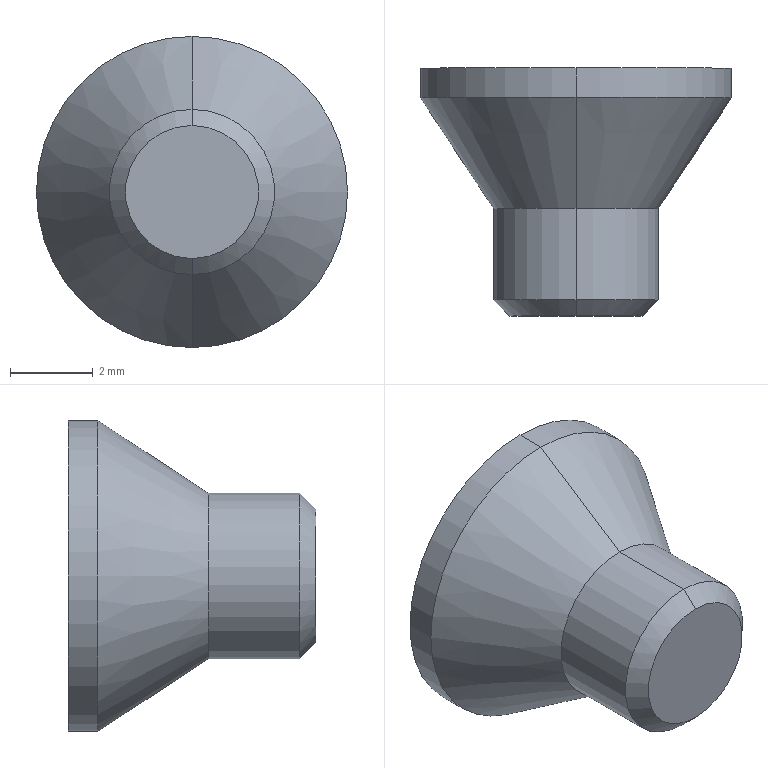Part | SolidWorks | features BaseBody 1 | 1 solid | 17 faces | box 7.53 x 6 x 7.53 mm | volume 127.383 mm3 | plane 9 | cone 4 | cylinder 4 | commonest cylinder face diameters 4 x2 7.53 x2
STEP:
#1=CARTESIAN_POINT('',(0.,-2.6,-1.61));
#2=VERTEX_POINT('',#1);
#3=CARTESIAN_POINT('',(0.,-2.6,1.61));
#4=VERTEX_POINT('',#3);
#5=CARTESIAN_POINT('',(0.,-2.6,0.));
#6=DIRECTION('',(0.,-1.,0.));
#7=DIRECTION('',(0.,0.,-1.));
#8=AXIS2_PLACEMENT_3D('',#5,#6,#7);
#9=CIRCLE('',#8,1.61);
#10=EDGE_CURVE('',#2,#4,#9,.T.);
#11=ORIENTED_EDGE('',*,*,#10,.F.);
#12=CARTESIAN_POINT('',(0.,-2.21,-2.));
#13=VERTEX_POINT('',#12);
#14=CARTESIAN_POINT('',(0.,-2.6,-1.61));
#15=DIRECTION('',(0.,0.7071,-0.7071));
#16=VECTOR('',#15,1000.);
#17=LINE('',#14,#16);
#18=EDGE_CURVE('',#2,#13,#17,.T.);
#19=ORIENTED_EDGE('',*,*,#18,.T.);
#20=CARTESIAN_POINT('',(0.,-2.21,2.));
#21=VERTEX_POINT('',#20);
#22=CARTESIAN_POINT('',(0.,-2.21,0.));
#23=DIRECTION('',(0.,1.,0.));
#24=DIRECTION('',(0.,0.,-1.));
#25=AXIS2_PLACEMENT_3D('',#22,#23,#24);
#26=CIRCLE('',#25,2.);
#27=EDGE_CURVE('',#21,#13,#26,.T.);
#28=ORIENTED_EDGE('',*,*,#27,.F.);
#29=CARTESIAN_POINT('',(0.,-2.6,1.61));
#30=DIRECTION('',(0.,0.7071,0.7071));
#31=VECTOR('',#30,1000.);
#32=LINE('',#29,#31);
#33=EDGE_CURVE('',#4,#21,#32,.T.);
#34=ORIENTED_EDGE('',*,*,#33,.F.);
#35=EDGE_LOOP('',(#11,#19,#28,#34));
#36=FACE_OUTER_BOUND('',#35,.T.);
#37=CARTESIAN_POINT('',(0.,-2.6,0.));
#38=DIRECTION('',(0.,1.,0.));
#39=DIRECTION('',(0.,0.,1.));
#40=AXIS2_PLACEMENT_3D('',#37,#38,#39);
#41=CONICAL_SURFACE('',#40,1.61,0.7854);
#42=ADVANCED_FACE('',(#36),#41,.T.);
#43=ORIENTED_EDGE('',*,*,#27,.T.);
#44=CARTESIAN_POINT('',(0.,0.,-2.));
#45=VERTEX_POINT('',#44);
#46=CARTESIAN_POINT('',(0.,-2.6,-2.));
#47=DIRECTION('',(0.,1.,0.));
#48=VECTOR('',#47,1000.);
#49=LINE('',#46,#48);
#50=EDGE_CURVE('',#13,#45,#49,.T.);
#51=ORIENTED_EDGE('',*,*,#50,.T.);
#52=CARTESIAN_POINT('',(0.,0.,2.));
#53=VERTEX_POINT('',#52);
#54=CARTESIAN_POINT('',(0.,0.,0.));
#55=DIRECTION('',(0.,1.,0.));
#56=DIRECTION('',(0.,0.,1.));
#57=AXIS2_PLACEMENT_3D('',#54,#55,#56);
#58=CIRCLE('',#57,2.);
#59=EDGE_CURVE('',#53,#45,#58,.T.);
#60=ORIENTED_EDGE('',*,*,#59,.F.);
#61=CARTESIAN_POINT('',(0.,-2.6,2.));
#62=DIRECTION('',(0.,1.,0.));
#63=VECTOR('',#62,1000.);
#64=LINE('',#61,#63);
#65=EDGE_CURVE('',#21,#53,#64,.T.);
#66=ORIENTED_EDGE('',*,*,#65,.F.);
#67=EDGE_LOOP('',(#43,#51,#60,#66));
#68=FACE_OUTER_BOUND('',#67,.T.);
#69=CARTESIAN_POINT('',(0.,-2.6,0.));
#70=DIRECTION('',(0.,1.,0.));
#71=DIRECTION('',(0.,0.,1.));
#72=AXIS2_PLACEMENT_3D('',#69,#70,#71);
#73=CYLINDRICAL_SURFACE('',#72,2.);
#74=ADVANCED_FACE('',(#68),#73,.T.);
#75=ORIENTED_EDGE('',*,*,#59,.T.);
#76=CARTESIAN_POINT('',(0.,2.685,-3.765));
#77=VERTEX_POINT('',#76);
#78=CARTESIAN_POINT('',(0.,2.685,-3.765));
#79=DIRECTION('',(0.,0.8356,-0.5493));
#80=VECTOR('',#79,1000.);
#81=LINE('',#78,#80);
#82=EDGE_CURVE('',#45,#77,#81,.T.);
#83=ORIENTED_EDGE('',*,*,#82,.T.);
#84=CARTESIAN_POINT('',(0.,2.685,3.765));
#85=VERTEX_POINT('',#84);
#86=CARTESIAN_POINT('',(0.,2.685,0.));
#87=DIRECTION('',(0.,1.,0.));
#88=DIRECTION('',(0.,0.,1.));
#89=AXIS2_PLACEMENT_3D('',#86,#87,#88);
#90=CIRCLE('',#89,3.765);
#91=EDGE_CURVE('',#85,#77,#90,.T.);
#92=ORIENTED_EDGE('',*,*,#91,.F.);
#93=CARTESIAN_POINT('',(0.,2.685,3.765));
#94=DIRECTION('',(0.,0.8356,0.5493));
#95=VECTOR('',#94,1000.);
#96=LINE('',#93,#95);
#97=EDGE_CURVE('',#53,#85,#96,.T.);
#98=ORIENTED_EDGE('',*,*,#97,.F.);
#99=EDGE_LOOP('',(#75,#83,#92,#98));
#100=FACE_OUTER_BOUND('',#99,.T.);
#101=CARTESIAN_POINT('',(0.,2.685,0.));
#102=DIRECTION('',(0.,1.,0.));
#103=DIRECTION('',(0.,0.,1.));
#104=AXIS2_PLACEMENT_3D('',#101,#102,#103);
#105=CONICAL_SURFACE('',#104,3.765,0.5815);
#106=ADVANCED_FACE('',(#100),#105,.T.);
#107=CARTESIAN_POINT('',(0.,3.4,3.765));
#108=VERTEX_POINT('',#107);
#109=CARTESIAN_POINT('',(0.,3.4,-3.765));
#110=VERTEX_POINT('',#109);
#111=CARTESIAN_POINT('',(0.,3.4,0.));
#112=DIRECTION('',(0.,1.,0.));
#113=DIRECTION('',(0.,0.,1.));
#114=AXIS2_PLACEMENT_3D('',#111,#112,#113);
#115=CIRCLE('',#114,3.765);
#116=EDGE_CURVE('',#108,#110,#115,.T.);
#117=ORIENTED_EDGE('',*,*,#116,.F.);
#118=CARTESIAN_POINT('',(0.,3.4,3.765));
#119=DIRECTION('',(0.,-1.,0.));
#120=VECTOR('',#119,1000.);
#121=LINE('',#118,#120);
#122=EDGE_CURVE('',#108,#85,#121,.T.);
#123=ORIENTED_EDGE('',*,*,#122,.T.);
#124=ORIENTED_EDGE('',*,*,#91,.T.);
#125=CARTESIAN_POINT('',(0.,3.4,-3.765));
#126=DIRECTION('',(0.,-1.,0.));
#127=VECTOR('',#126,1000.);
#128=LINE('',#125,#127);
#129=EDGE_CURVE('',#110,#77,#128,.T.);
#130=ORIENTED_EDGE('',*,*,#129,.F.);
#131=EDGE_LOOP('',(#117,#123,#124,#130));
#132=FACE_OUTER_BOUND('',#131,.T.);
#133=CARTESIAN_POINT('',(0.,3.4,0.));
#134=DIRECTION('',(0.,-1.,0.));
#135=DIRECTION('',(0.,0.,-1.));
#136=AXIS2_PLACEMENT_3D('',#133,#134,#135);
#137=CYLINDRICAL_SURFACE('',#136,3.765);
#138=ADVANCED_FACE('',(#132),#137,.T.);
#139=CARTESIAN_POINT('',(0.,-2.6,0.));
#140=DIRECTION('',(0.,-1.,0.));
#141=DIRECTION('',(0.,0.,-1.));
#142=AXIS2_PLACEMENT_3D('',#139,#140,#141);
#143=CIRCLE('',#142,1.61);
#144=EDGE_CURVE('',#4,#2,#143,.T.);
#145=ORIENTED_EDGE('',*,*,#144,.T.);
#146=ORIENTED_EDGE('',*,*,#10,.T.);
#147=EDGE_LOOP('',(#145,#146));
#148=FACE_OUTER_BOUND('',#147,.T.);
#149=CARTESIAN_POINT('',(0.,-2.6,0.));
#150=DIRECTION('',(0.,-1.,0.));
#151=DIRECTION('',(0.,0.,-1.));
#152=AXIS2_PLACEMENT_3D('',#149,#150,#151);
#153=PLANE('',#152);
#154=ADVANCED_FACE('',(#148),#153,.T.);
#155=CARTESIAN_POINT('',(0.739,1.9,1.28));
#156=VERTEX_POINT('',#155);
#157=CARTESIAN_POINT('',(1.478,1.9,0.));
#158=VERTEX_POINT('',#157);
#159=CARTESIAN_POINT('',(0.739,1.9,1.28));
#160=DIRECTION('',(0.5,0.,-0.866));
#161=VECTOR('',#160,1000.);
#162=LINE('',#159,#161);
#163=EDGE_CURVE('',#156,#158,#162,.T.);
#164=ORIENTED_EDGE('',*,*,#163,.T.);
#165=CARTESIAN_POINT('',(0.739,1.9,-1.28));
#166=VERTEX_POINT('',#165);
#167=CARTESIAN_POINT('',(1.478,1.9,0.));
#168=DIRECTION('',(-0.5,0.,-0.866));
#169=VECTOR('',#168,1000.);
#170=LINE('',#167,#169);
#171=EDGE_CURVE('',#158,#166,#170,.T.);
#172=ORIENTED_EDGE('',*,*,#171,.T.);
#173=CARTESIAN_POINT('',(-0.739,1.9,-1.28));
#174=VERTEX_POINT('',#173);
#175=CARTESIAN_POINT('',(0.739,1.9,-1.28));
#176=DIRECTION('',(-1.,0.,0.));
#177=VECTOR('',#176,1000.);
#178=LINE('',#175,#177);
#179=EDGE_CURVE('',#166,#174,#178,.T.);
#180=ORIENTED_EDGE('',*,*,#179,.T.);
#181=CARTESIAN_POINT('',(-1.478,1.9,0.));
#182=VERTEX_POINT('',#181);
#183=CARTESIAN_POINT('',(-0.739,1.9,-1.28));
#184=DIRECTION('',(-0.5,0.,0.866));
#185=VECTOR('',#184,1000.);
#186=LINE('',#183,#185);
#187=EDGE_CURVE('',#174,#182,#186,.T.);
#188=ORIENTED_EDGE('',*,*,#187,.T.);
#189=CARTESIAN_POINT('',(-0.739,1.9,1.28));
#190=VERTEX_POINT('',#189);
#191=CARTESIAN_POINT('',(-1.478,1.9,0.));
#192=DIRECTION('',(0.5,0.,0.866));
#193=VECTOR('',#192,1000.);
#194=LINE('',#191,#193);
#195=EDGE_CURVE('',#182,#190,#194,.T.);
#196=ORIENTED_EDGE('',*,*,#195,.T.);
#197=CARTESIAN_POINT('',(-0.739,1.9,1.28));
#198=DIRECTION('',(1.,0.,0.));
#199=VECTOR('',#198,1000.);
#200=LINE('',#197,#199);
#201=EDGE_CURVE('',#190,#156,#200,.T.);
#202=ORIENTED_EDGE('',*,*,#201,.T.);
#203=EDGE_LOOP('',(#164,#172,#180,#188,#196,#202));
#204=FACE_OUTER_BOUND('',#203,.T.);
#205=CARTESIAN_POINT('',(0.,1.9,0.));
#206=DIRECTION('',(0.,1.,0.));
#207=DIRECTION('',(1.,0.,0.));
#208=AXIS2_PLACEMENT_3D('',#205,#206,#207);
#209=PLANE('',#208);
#210=ADVANCED_FACE('',(#204),#209,.T.);
#211=CARTESIAN_POINT('',(1.478,3.4,0.));
#212=VERTEX_POINT('',#211);
#213=CARTESIAN_POINT('',(0.739,3.4,-1.28));
#214=VERTEX_POINT('',#213);
#215=CARTESIAN_POINT('',(1.478,3.4,0.));
#216=DIRECTION('',(-0.5,0.,-0.866));
#217=VECTOR('',#216,1000.);
#218=LINE('',#215,#217);
#219=EDGE_CURVE('',#212,#214,#218,.T.);
#220=ORIENTED_EDGE('',*,*,#219,.T.);
#221=CARTESIAN_POINT('',(0.739,1.9,-1.28));
#222=DIRECTION('',(0.,1.,0.));
#223=VECTOR('',#222,1000.);
#224=LINE('',#221,#223);
#225=EDGE_CURVE('',#166,#214,#224,.T.);
#226=ORIENTED_EDGE('',*,*,#225,.F.);
#227=ORIENTED_EDGE('',*,*,#171,.F.);
#228=CARTESIAN_POINT('',(1.478,1.9,0.));
#229=DIRECTION('',(0.,1.,0.));
#230=VECTOR('',#229,1000.);
#231=LINE('',#228,#230);
#232=EDGE_CURVE('',#158,#212,#231,.T.);
#233=ORIENTED_EDGE('',*,*,#232,.T.);
#234=EDGE_LOOP('',(#220,#226,#227,#233));
#235=FACE_OUTER_BOUND('',#234,.T.);
#236=CARTESIAN_POINT('',(1.478,1.9,0.));
#237=DIRECTION('',(0.866,0.,-0.5));
#238=DIRECTION('',(0.,-1.,0.));
#239=AXIS2_PLACEMENT_3D('',#236,#237,#238);
#240=PLANE('',#239);
#241=ADVANCED_FACE('',(#235),#240,.F.);
#242=CARTESIAN_POINT('',(-0.739,3.4,-1.28));
#243=VERTEX_POINT('',#242);
#244=CARTESIAN_POINT('',(0.739,3.4,-1.28));
#245=DIRECTION('',(-1.,0.,0.));
#246=VECTOR('',#245,1000.);
#247=LINE('',#244,#246);
#248=EDGE_CURVE('',#214,#243,#247,.T.);
#249=ORIENTED_EDGE('',*,*,#248,.T.);
#250=CARTESIAN_POINT('',(-0.739,1.9,-1.28));
#251=DIRECTION('',(0.,1.,0.));
#252=VECTOR('',#251,1000.);
#253=LINE('',#250,#252);
#254=EDGE_CURVE('',#174,#243,#253,.T.);
#255=ORIENTED_EDGE('',*,*,#254,.F.);
#256=ORIENTED_EDGE('',*,*,#179,.F.);
#257=ORIENTED_EDGE('',*,*,#225,.T.);
#258=EDGE_LOOP('',(#249,#255,#256,#257));
#259=FACE_OUTER_BOUND('',#258,.T.);
#260=CARTESIAN_POINT('',(0.739,1.9,-1.28));
#261=DIRECTION('',(0.,0.,-1.));
#262=DIRECTION('',(0.,-1.,0.));
#263=AXIS2_PLACEMENT_3D('',#260,#261,#262);
#264=PLANE('',#263);
#265=ADVANCED_FACE('',(#259),#264,.F.);
#266=CARTESIAN_POINT('',(-1.478,3.4,0.));
#267=VERTEX_POINT('',#266);
#268=CARTESIAN_POINT('',(-0.739,3.4,-1.28));
#269=DIRECTION('',(-0.5,0.,0.866));
#270=VECTOR('',#269,1000.);
#271=LINE('',#268,#270);
#272=EDGE_CURVE('',#243,#267,#271,.T.);
#273=ORIENTED_EDGE('',*,*,#272,.T.);
#274=CARTESIAN_POINT('',(-1.478,1.9,0.));
#275=DIRECTION('',(0.,1.,0.));
#276=VECTOR('',#275,1000.);
#277=LINE('',#274,#276);
#278=EDGE_CURVE('',#182,#267,#277,.T.);
#279=ORIENTED_EDGE('',*,*,#278,.F.);
#280=ORIENTED_EDGE('',*,*,#187,.F.);
#281=ORIENTED_EDGE('',*,*,#254,.T.);
#282=EDGE_LOOP('',(#273,#279,#280,#281));
#283=FACE_OUTER_BOUND('',#282,.T.);
#284=CARTESIAN_POINT('',(-0.739,1.9,-1.28));
#285=DIRECTION('',(-0.866,0.,-0.5));
#286=DIRECTION('',(-0.5,0.,0.866));
#287=AXIS2_PLACEMENT_3D('',#284,#285,#286);
#288=PLANE('',#287);
#289=ADVANCED_FACE('',(#283),#288,.F.);
#290=CARTESIAN_POINT('',(-0.739,3.4,1.28));
#291=VERTEX_POINT('',#290);
#292=CARTESIAN_POINT('',(-1.478,3.4,0.));
#293=DIRECTION('',(0.5,0.,0.866));
#294=VECTOR('',#293,1000.);
#295=LINE('',#292,#294);
#296=EDGE_CURVE('',#267,#291,#295,.T.);
#297=ORIENTED_EDGE('',*,*,#296,.T.);
#298=CARTESIAN_POINT('',(-0.739,1.9,1.28));
#299=DIRECTION('',(0.,1.,0.));
#300=VECTOR('',#299,1000.);
#301=LINE('',#298,#300);
#302=EDGE_CURVE('',#190,#291,#301,.T.);
#303=ORIENTED_EDGE('',*,*,#302,.F.);
#304=ORIENTED_EDGE('',*,*,#195,.F.);
#305=ORIENTED_EDGE('',*,*,#278,.T.);
#306=EDGE_LOOP('',(#297,#303,#304,#305));
#307=FACE_OUTER_BOUND('',#306,.T.);
#308=CARTESIAN_POINT('',(-1.478,1.9,0.));
#309=DIRECTION('',(-0.866,0.,0.5));
#310=DIRECTION('',(0.,1.,0.));
#311=AXIS2_PLACEMENT_3D('',#308,#309,#310);
#312=PLANE('',#311);
#313=ADVANCED_FACE('',(#307),#312,.F.);
#314=CARTESIAN_POINT('',(0.739,3.4,1.28));
#315=VERTEX_POINT('',#314);
#316=CARTESIAN_POINT('',(-0.739,3.4,1.28));
#317=DIRECTION('',(1.,0.,0.));
#318=VECTOR('',#317,1000.);
#319=LINE('',#316,#318);
#320=EDGE_CURVE('',#291,#315,#319,.T.);
#321=ORIENTED_EDGE('',*,*,#320,.T.);
#322=CARTESIAN_POINT('',(0.739,1.9,1.28));
#323=DIRECTION('',(0.,1.,0.));
#324=VECTOR('',#323,1000.);
#325=LINE('',#322,#324);
#326=EDGE_CURVE('',#156,#315,#325,.T.);
#327=ORIENTED_EDGE('',*,*,#326,.F.);
#328=ORIENTED_EDGE('',*,*,#201,.F.);
#329=ORIENTED_EDGE('',*,*,#302,.T.);
#330=EDGE_LOOP('',(#321,#327,#328,#329));
#331=FACE_OUTER_BOUND('',#330,.T.);
#332=CARTESIAN_POINT('',(-0.739,1.9,1.28));
#333=DIRECTION('',(0.,0.,1.));
#334=DIRECTION('',(1.,0.,0.));
#335=AXIS2_PLACEMENT_3D('',#332,#333,#334);
#336=PLANE('',#335);
#337=ADVANCED_FACE('',(#331),#336,.F.);
#338=CARTESIAN_POINT('',(0.739,3.4,1.28));
#339=DIRECTION('',(0.5,0.,-0.866));
#340=VECTOR('',#339,1000.);
#341=LINE('',#338,#340);
#342=EDGE_CURVE('',#315,#212,#341,.T.);
#343=ORIENTED_EDGE('',*,*,#342,.T.);
#344=ORIENTED_EDGE('',*,*,#232,.F.);
#345=ORIENTED_EDGE('',*,*,#163,.F.);
#346=ORIENTED_EDGE('',*,*,#326,.T.);
#347=EDGE_LOOP('',(#343,#344,#345,#346));
#348=FACE_OUTER_BOUND('',#347,.T.);
#349=CARTESIAN_POINT('',(0.739,1.9,1.28));
#350=DIRECTION('',(0.866,0.,0.5));
#351=DIRECTION('',(0.,-1.,0.));
#352=AXIS2_PLACEMENT_3D('',#349,#350,#351);
#353=PLANE('',#352);
#354=ADVANCED_FACE('',(#348),#353,.F.);
#355=ORIENTED_EDGE('',*,*,#342,.F.);
#356=ORIENTED_EDGE('',*,*,#320,.F.);
#357=ORIENTED_EDGE('',*,*,#296,.F.);
#358=ORIENTED_EDGE('',*,*,#272,.F.);
#359=ORIENTED_EDGE('',*,*,#248,.F.);
#360=ORIENTED_EDGE('',*,*,#219,.F.);
#361=EDGE_LOOP('',(#355,#356,#357,#358,#359,#360));
#362=FACE_BOUND('',#361,.T.);
#363=CARTESIAN_POINT('',(0.,3.4,0.));
#364=DIRECTION('',(0.,1.,0.));
#365=DIRECTION('',(0.,0.,1.));
#366=AXIS2_PLACEMENT_3D('',#363,#364,#365);
#367=CIRCLE('',#366,3.765);
#368=EDGE_CURVE('',#110,#108,#367,.T.);
#369=ORIENTED_EDGE('',*,*,#368,.T.);
#370=ORIENTED_EDGE('',*,*,#116,.T.);
#371=EDGE_LOOP('',(#369,#370));
#372=FACE_OUTER_BOUND('',#371,.T.);
#373=CARTESIAN_POINT('',(0.,3.4,0.));
#374=DIRECTION('',(0.,1.,0.));
#375=DIRECTION('',(1.,0.,0.));
#376=AXIS2_PLACEMENT_3D('',#373,#374,#375);
#377=PLANE('',#376);
#378=ADVANCED_FACE('',(#362,#372),#377,.T.);
#379=ORIENTED_EDGE('',*,*,#122,.F.);
#380=ORIENTED_EDGE('',*,*,#368,.F.);
#381=ORIENTED_EDGE('',*,*,#129,.T.);
#382=CARTESIAN_POINT('',(0.,2.685,0.));
#383=DIRECTION('',(0.,1.,0.));
#384=DIRECTION('',(0.,0.,1.));
#385=AXIS2_PLACEMENT_3D('',#382,#383,#384);
#386=CIRCLE('',#385,3.765);
#387=EDGE_CURVE('',#77,#85,#386,.T.);
#388=ORIENTED_EDGE('',*,*,#387,.T.);
#389=EDGE_LOOP('',(#379,#380,#381,#388));
#390=FACE_OUTER_BOUND('',#389,.T.);
#391=CARTESIAN_POINT('',(0.,3.4,0.));
#392=DIRECTION('',(0.,-1.,0.));
#393=DIRECTION('',(0.,0.,-1.));
#394=AXIS2_PLACEMENT_3D('',#391,#392,#393);
#395=CYLINDRICAL_SURFACE('',#394,3.765);
#396=ADVANCED_FACE('',(#390),#395,.T.);
#397=ORIENTED_EDGE('',*,*,#82,.F.);
#398=CARTESIAN_POINT('',(0.,0.,0.));
#399=DIRECTION('',(0.,1.,0.));
#400=DIRECTION('',(0.,0.,1.));
#401=AXIS2_PLACEMENT_3D('',#398,#399,#400);
#402=CIRCLE('',#401,2.);
#403=EDGE_CURVE('',#45,#53,#402,.T.);
#404=ORIENTED_EDGE('',*,*,#403,.T.);
#405=ORIENTED_EDGE('',*,*,#97,.T.);
#406=ORIENTED_EDGE('',*,*,#387,.F.);
#407=EDGE_LOOP('',(#397,#404,#405,#406));
#408=FACE_OUTER_BOUND('',#407,.T.);
#409=CARTESIAN_POINT('',(0.,2.685,0.));
#410=DIRECTION('',(0.,1.,0.));
#411=DIRECTION('',(0.,0.,1.));
#412=AXIS2_PLACEMENT_3D('',#409,#410,#411);
#413=CONICAL_SURFACE('',#412,3.765,0.5815);
#414=ADVANCED_FACE('',(#408),#413,.T.);
#415=ORIENTED_EDGE('',*,*,#50,.F.);
#416=CARTESIAN_POINT('',(0.,-2.21,0.));
#417=DIRECTION('',(0.,1.,0.));
#418=DIRECTION('',(0.,0.,-1.));
#419=AXIS2_PLACEMENT_3D('',#416,#417,#418);
#420=CIRCLE('',#419,2.);
#421=EDGE_CURVE('',#13,#21,#420,.T.);
#422=ORIENTED_EDGE('',*,*,#421,.T.);
#423=ORIENTED_EDGE('',*,*,#65,.T.);
#424=ORIENTED_EDGE('',*,*,#403,.F.);
#425=EDGE_LOOP('',(#415,#422,#423,#424));
#426=FACE_OUTER_BOUND('',#425,.T.);
#427=CARTESIAN_POINT('',(0.,-2.6,0.));
#428=DIRECTION('',(0.,1.,0.));
#429=DIRECTION('',(0.,0.,1.));
#430=AXIS2_PLACEMENT_3D('',#427,#428,#429);
#431=CYLINDRICAL_SURFACE('',#430,2.);
#432=ADVANCED_FACE('',(#426),#431,.T.);
#433=ORIENTED_EDGE('',*,*,#18,.F.);
#434=ORIENTED_EDGE('',*,*,#144,.F.);
#435=ORIENTED_EDGE('',*,*,#33,.T.);
#436=ORIENTED_EDGE('',*,*,#421,.F.);
#437=EDGE_LOOP('',(#433,#434,#435,#436));
#438=FACE_OUTER_BOUND('',#437,.T.);
#439=CARTESIAN_POINT('',(0.,-2.6,0.));
#440=DIRECTION('',(0.,1.,0.));
#441=DIRECTION('',(0.,0.,1.));
#442=AXIS2_PLACEMENT_3D('',#439,#440,#441);
#443=CONICAL_SURFACE('',#442,1.61,0.7854);
#444=ADVANCED_FACE('',(#438),#443,.T.);
#445=CLOSED_SHELL('',(#42,#74,#106,#138,#154,#210,#241,#265,#289,#313,#337,#354,#378,#396,#414,#432,#444));
#446=MANIFOLD_SOLID_BREP('',#445);
#447=CARTESIAN_POINT('',(0.,0.,0.));
#448=DIRECTION('',(0.,0.,1.));
#449=DIRECTION('',(1.,0.,0.));
#450=AXIS2_PLACEMENT_3D('',#447,#448,#449);
#451=(LENGTH_UNIT()NAMED_UNIT(*)SI_UNIT(.MILLI.,.METRE.));
#452=UNCERTAINTY_MEASURE_WITH_UNIT(LENGTH_MEASURE(0.00001),#451,'','');
#453=(NAMED_UNIT(*)PLANE_ANGLE_UNIT()SI_UNIT($,.RADIAN.));
#454=(NAMED_UNIT(*)SI_UNIT($,.STERADIAN.)SOLID_ANGLE_UNIT());
#455=(GEOMETRIC_REPRESENTATION_CONTEXT(3)GLOBAL_UNCERTAINTY_ASSIGNED_CONTEXT((#452))GLOBAL_UNIT_ASSIGNED_CONTEXT((#451,#453,#454))REPRESENTATION_CONTEXT('',''));
#456=ADVANCED_BREP_SHAPE_REPRESENTATION('',(#446,#450),#455);